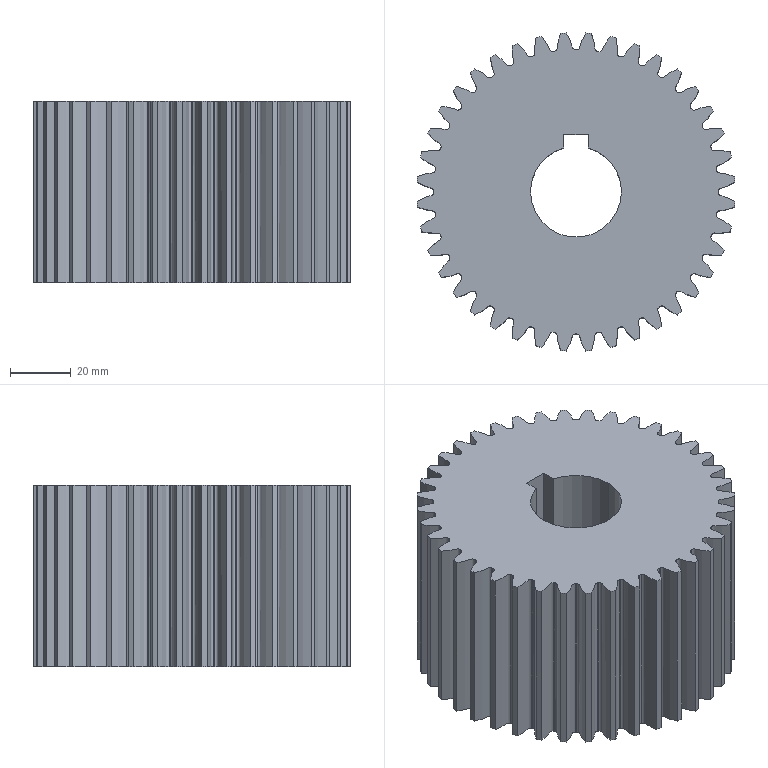Part | SolidWorks | features ICE 3, CirPattern 1, Extrusion 1, RefAxis 1 | 1 solid | 168 faces | box 104.808 x 104.808 x 60 mm | volume 422775 mm3 | cylinder 83 | spline 80 | plane 5 | commonest cylinder face diameters 93.75 x40 105 x40 30 x3